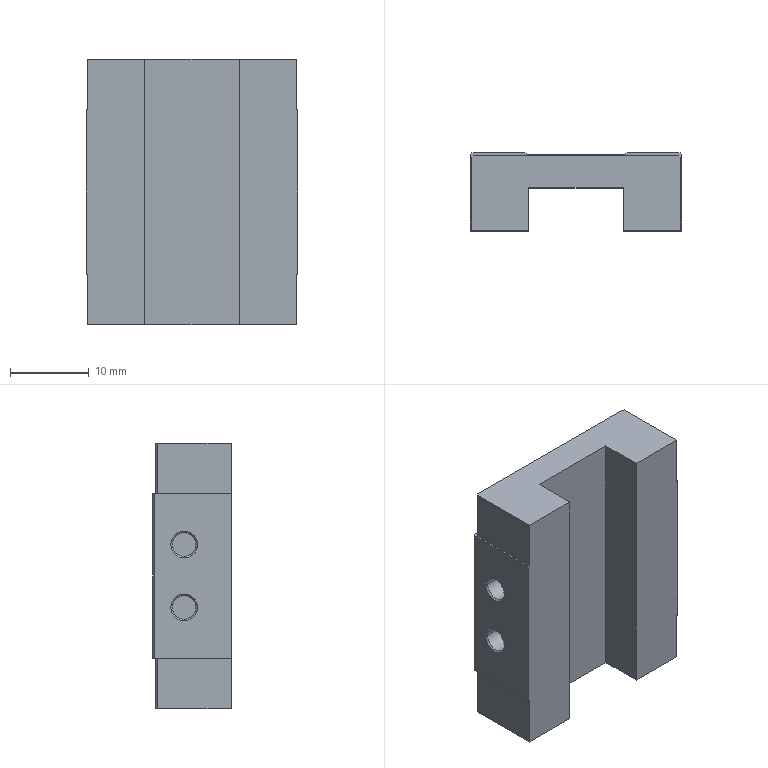Part | NX | 1 solid | 77 faces | box 27 x 10 x 33.8 mm | volume 6407 mm3 | plane 40 | cylinder 21 | cone 16 | commonest cylinder face diameters 3 x17 2 x4